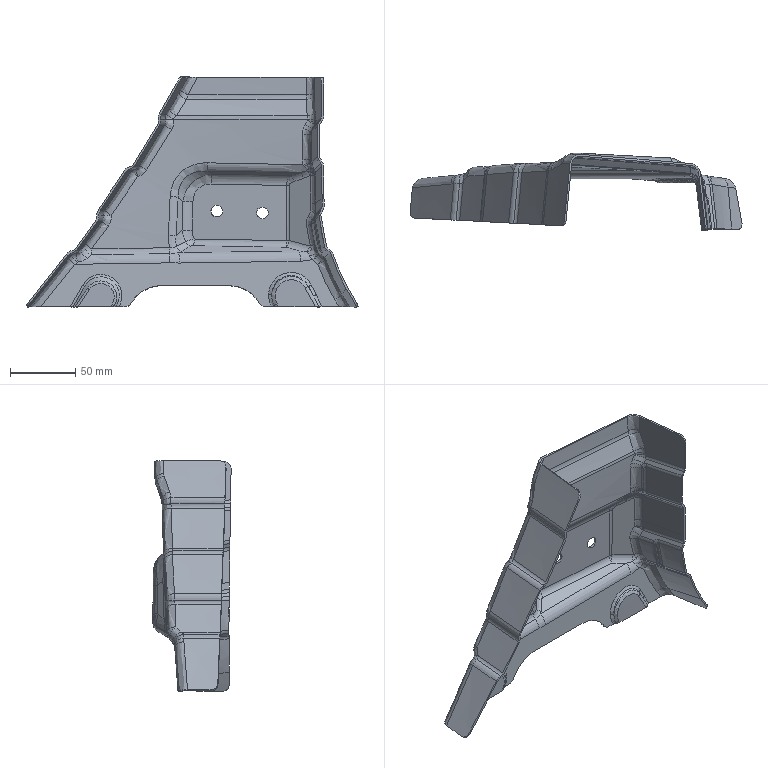Part | STEP file | FNA5401672 | 1 solid | 398 faces | box 254.233 x 59.892 x 176.91 mm | volume 65515 mm3 | spline 322 | cylinder 46 | other 13 | sphere 12 | plane 5 | commonest cylinder face diameters 9 x11 12 x10 15 x6 6 x5 20 x3 3 x2